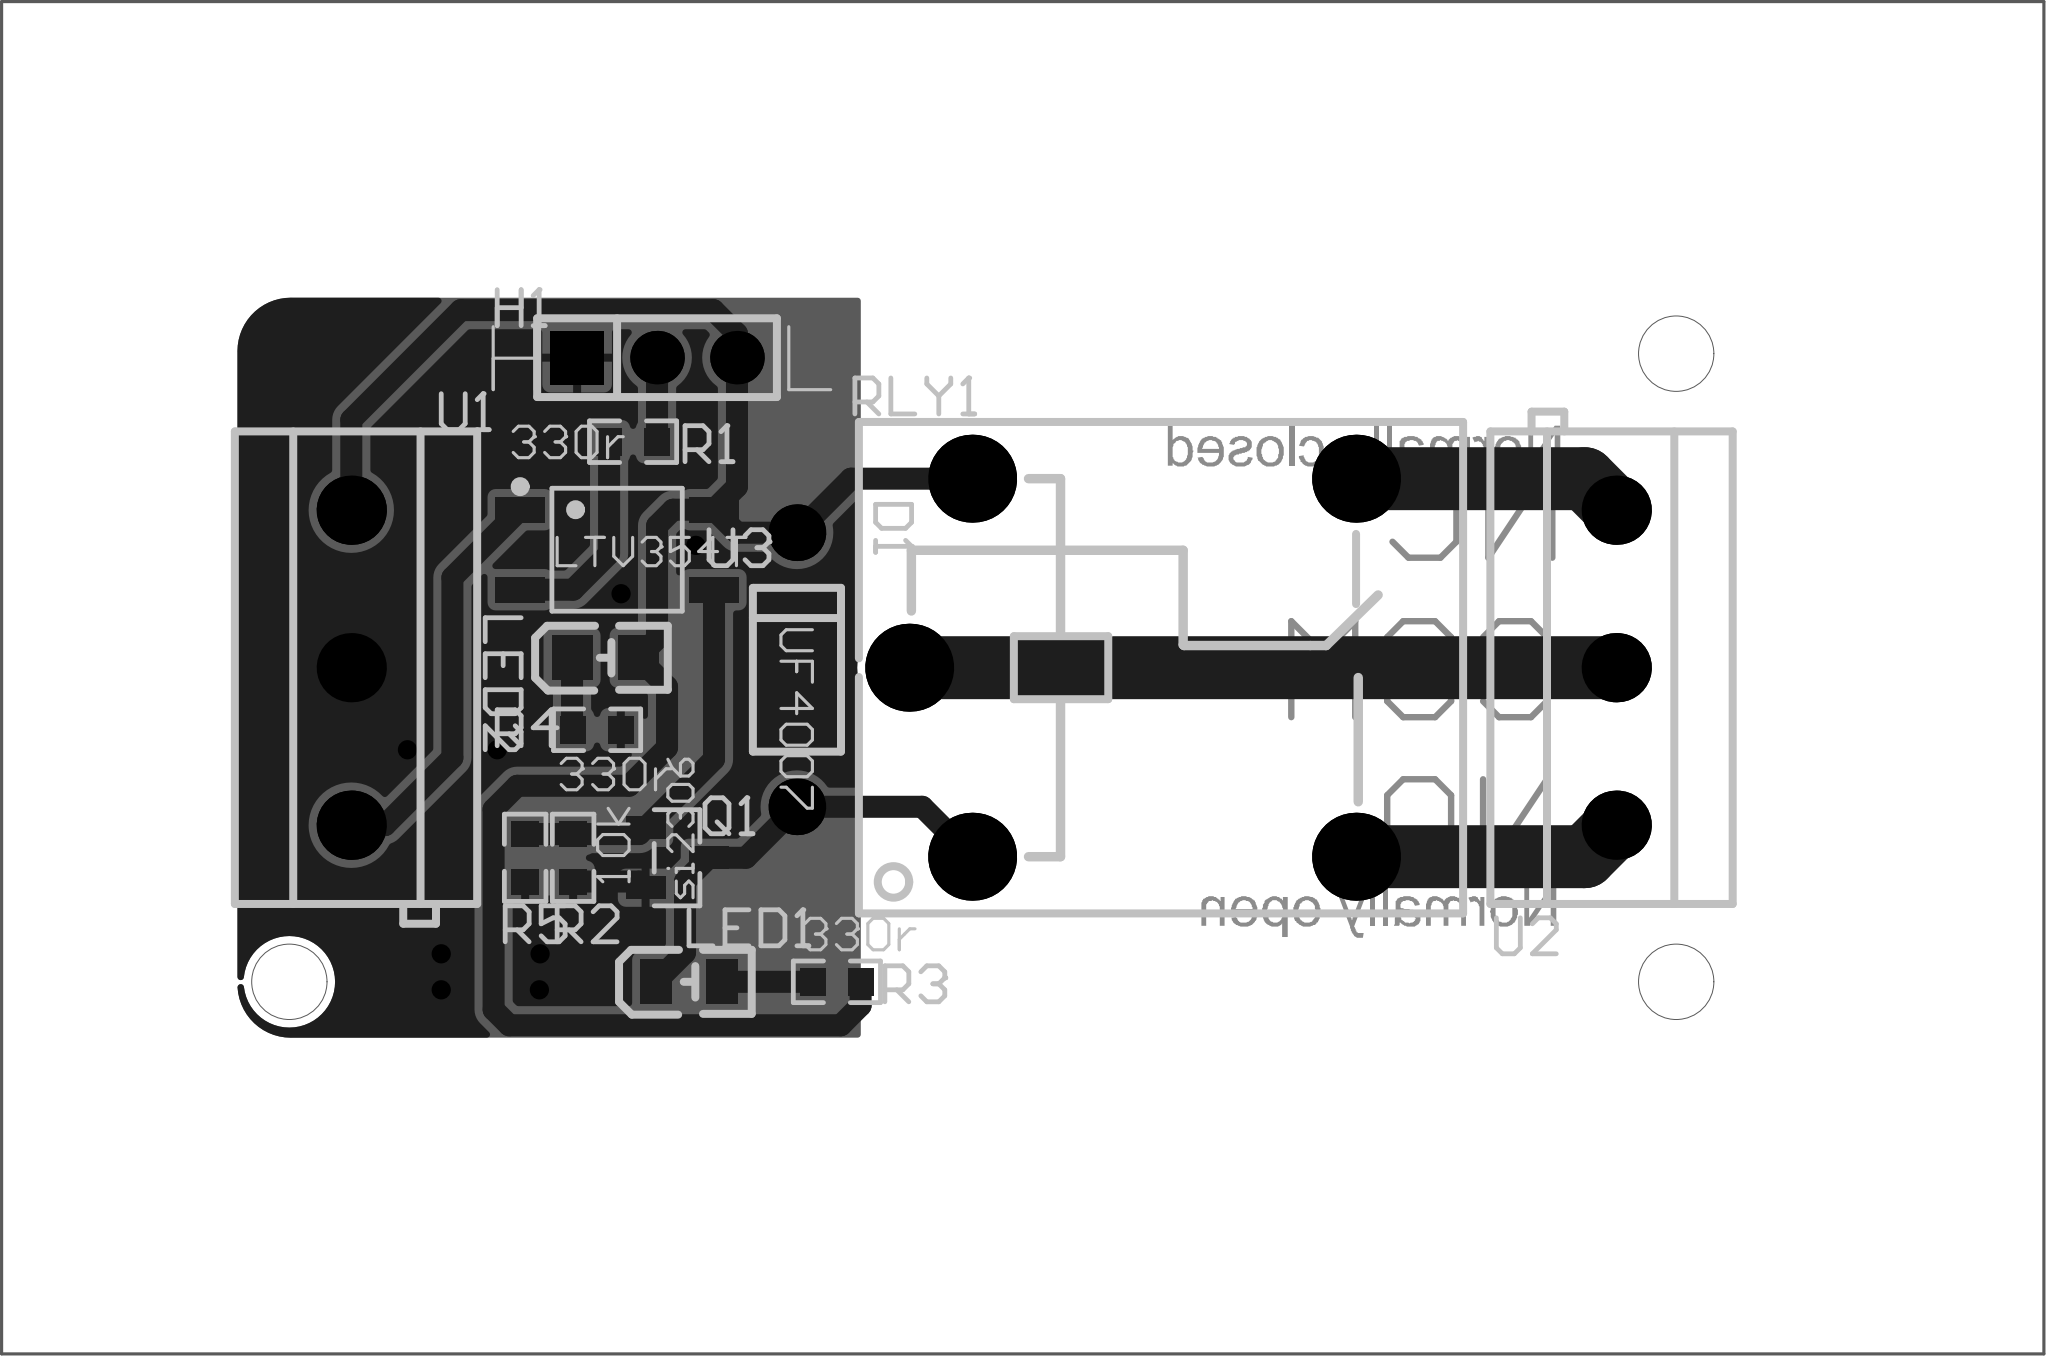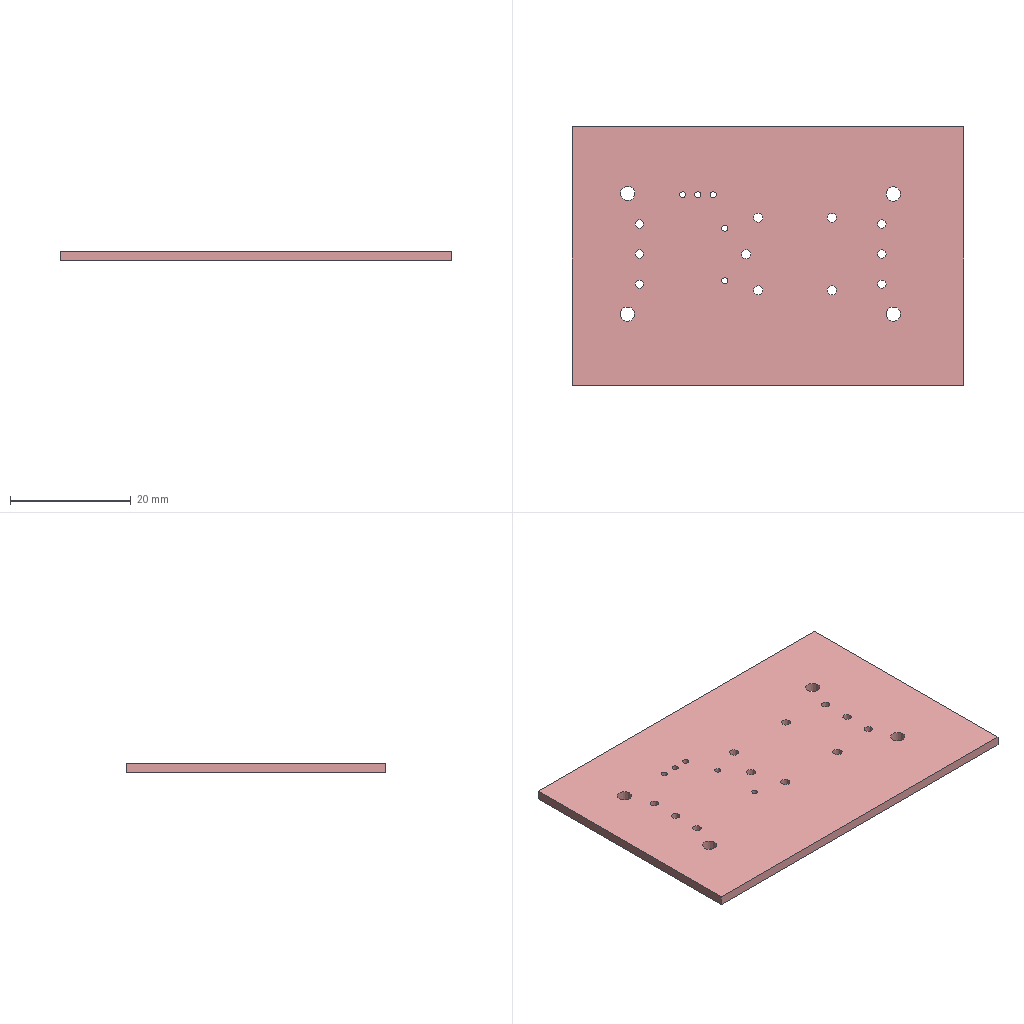Circuit board layout | Altium Designer | box 64.9 x 42.9 x 1.6 mm
Layer stack:
# Altium Designer layer stack of  (unit mm; dielectric type: 0 none, 1 core, 2 prepreg, 3 surface material)
index,name,kind,layer,copper_thickness_mm,dielectric_type,dielectric_thickness_mm,dielectric_material,dielectric_constant
0,Top Paste Mask Layer,other,,,,,,
1,Top Silkscreen Layer,other,,,,,,
2,Top Solder Mask Layer,dielectric,,,3,0.01,,3.3
3,Top Layer,copper,Top Layer,0.035,,,,
4,Dielectric1,dielectric,,,3,1.51,FR4,4.5
5,Bottom Layer,copper,Bottom Layer,0.035,,,,
6,Bottom Solder Mask Layer,dielectric,,,3,0.01,,3.3
7,Bottom Silkscreen Layer,other,,,,,,
8,Bottom Paste Mask Layer,other,,,,,,
# drill layer pairs: low layer,high layer
drill_pair,Top Layer,Bottom Layer
Part placement:
Designator,Comment,Layer,Footprint,Center-X(mm),Center-Y(mm),Rotation
U1,KF301-5.0-3P,TopLayer,CONN-TH_3P-P5.00_KF301-5.0-3P,80.962,91.632,270
H1,PZ254V-11-03P,TopLayer,HDR-TH_3P-P2.54-V-M_PZ254V-11-03P,90.678,101.473,0
D1,UF4007,TopLayer,DO-41_BD2.4-L4.7-P8.70-D0.9-RD,95.123,91.567,270
RLY1,SRD-05VDC-SL-C,TopLayer,RELAY-TH_SRD-XXVDC-XL-C,105.791,91.632,0
U2,KF301-5.0-3P,TopLayer,CONN-TH_3P-P5.00_KF301-5.0-3P,121.158,91.632,90
U3,LTV-354T-A,TopLayer,SOP-4_L3.9-W4.4-P2.54-LS7.0-TL,89.408,95.377,0
LED2,GL0805UG01,TopLayer,LED0805-FD_GL0805UG01,89.027,91.948,180
R2,10kΩ,TopLayer,R0603,88.011,85.598,90
R4,330Ω,TopLayer,R0603,88.773,89.662,0
R1,330Ω,TopLayer,R0603,89.916,98.806,180
Q1,SI2308A,TopLayer,SOT-23-3_L2.9-W1.3-P1.90-LS2.4-BR,91.313,85.598,180
LED1,GL0805UR01,TopLayer,LED0805-R-RD_RED,91.694,81.661,0
R3,330Ω,TopLayer,R0603,96.393,81.661,180
R5,10kΩ,TopLayer,R0603,86.487,85.598,270
Pad and via stacks:
# Altium Designer via and pad stacks of  (unit mm). Each distinct definition once, with the count of objects using it.
# via: kind,start_layer,end_layer,hole_mm,diameter_mm,mode(0 simple;1 top-mid-bottom;2 full stack),diameter_per_layer,count,example_net
# pad: kind,layer,hole_mm,hole_type(0 round;1 square;2 slot),plating,top_size,top_shape(1 round;2 rect;3 octagon;9 rounded rect),mid_size,bottom_size,mode,footprint,size_per_layer,count,example
pad,Multi-Layer,1.4,0,plated,2.2x2.2,1,2.2x2.2,2.2x2.2,0,CONN-TH_3P-P5.00_KF301-5.0-3P,,6,U1.1
pad,Multi-Layer,1.02,0,plated,1.7x1.7,2,1.7x1.7,1.7x1.7,0,HDR-TH_3P-P2.54-V-M_PZ254V-11-03P,,1,H1.1
pad,Multi-Layer,1.02,0,plated,1.7x1.7,1,1.7x1.7,1.7x1.7,0,HDR-TH_3P-P2.54-V-M_PZ254V-11-03P,,2,H1.2
pad,Multi-Layer,1,0,plated,1.8x1.8,1,1.8x1.8,1.8x1.8,0,DO-41_BD2.4-L4.7-P8.70-D0.9-RD,,2,D1.1
pad,Multi-Layer,1.524,0,plated,2.794x2.794,1,2.794x2.794,2.794x2.794,0,RELAY-TH_SRD-XXVDC-XL-C,,5,RLY1.2
pad,Top Layer,0,0,plated,1.56x0.8,2,1.56x0.8,1.56x0.8,0,SOP-4_L3.9-W4.4-P2.54-LS7.0-TL,,4,U3.1
pad,Top Layer,0,0,plated,1.3x1.399,2,1.3x1.399,1.3x1.399,0,LED0805-FD_GL0805UG01,,2,LED2.2
pad,Top Layer,0,0,plated,0.8065x0.864,2,0.8065x0.864,0.8065x0.864,0,R0603,,10,R2.2
pad,Top Layer,0,0,plated,1.25x0.7,2,1.25x0.7,1.25x0.7,0,SOT-23-3_L2.9-W1.3-P1.90-LS2.4-BR,,3,Q1.1
pad,Top Layer,0,0,plated,1x1.399,2,1x1.399,1x1.399,0,LED0805-R-RD_RED,,2,LED1.2
via,Top Layer,Bottom Layer,0.3048,0.61,0,,8,GND
Copper pours:
name,layer,net,type(0 solid;1 hatched;2 none)
Top Layer-GND,Top Layer,GND,0
Bottom Layer-GND,Bottom Layer,GND,0